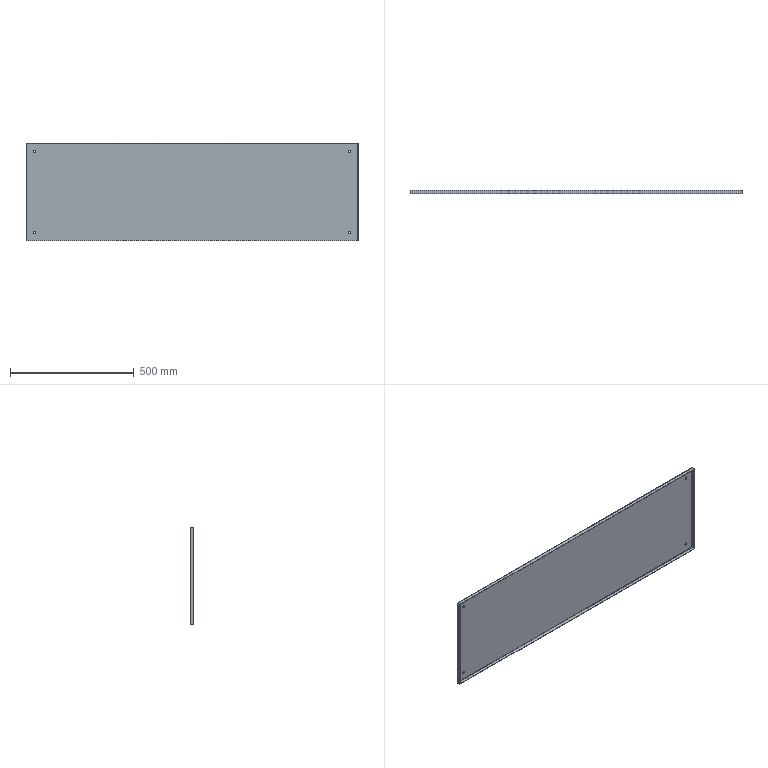Part | 1 solid | 46 faces | box 1340 x 15 x 395 mm | volume 860282 mm3 | plane 22 | cylinder 16 | spline 8 | commonest cylinder face diameters 10 x8 1.473 x4 4.473 x4